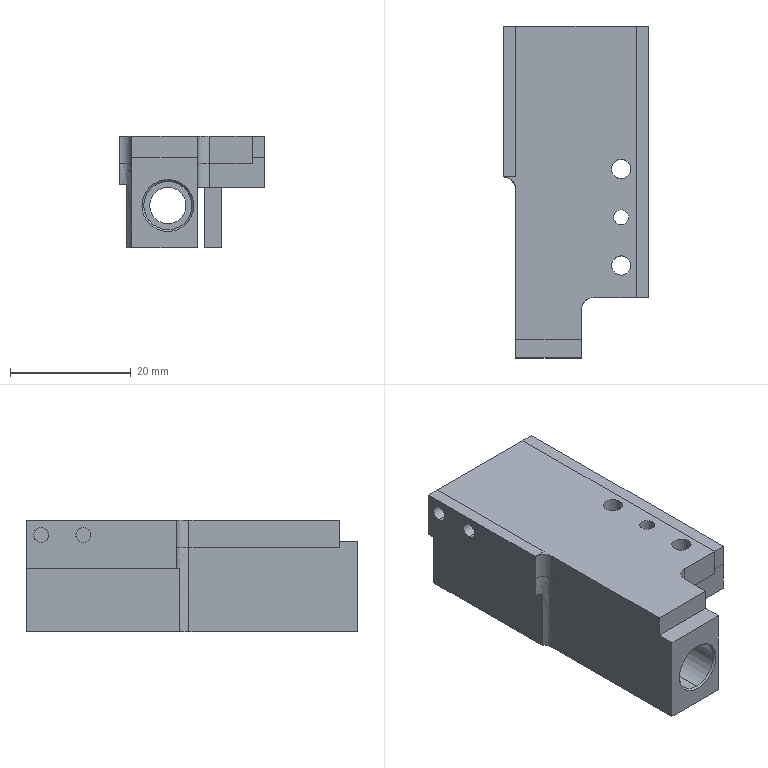NC program | NX | posted with a generic post | part box 24.15 x 55 x 18.5 mm
Whole program:
N10 G17 G21 G94 G90
(FLOOR_WALL_1_COPY_1_COPY , TOOL : D10)
N12 T10 M6
N14 G54
N16 G17 G0 G90 X18.075 Y6.103 B0. C0. S9500 M3
N18 G43 Z30. H10
N20 Z-0.85
N22 G94 G1 X17.575 Y5.815 F1000.
N24 G3 X17.075 Y4.949 R1.
N26 G1 Y-22.603 F3000.
N28 X6.003
N30 Y-32.5
N32 X-15.103
N34 Y-2.6
N36 X-4.9
N38 Y32.5
N40 X17.075
N42 Y4.949
N44 X12.075
N46 Y-17.603
N48 X6.003
N50 G3 X1.003 Y-22.603 R5.
N52 G1 Y-27.5
N54 X-10.103
N56 Y-7.6
N58 X-4.9
N60 G3 X0.1 Y-2.6 R5.
N62 G1 Y27.5
N64 X12.075
N66 Y4.949
N68 X7.075
N70 Y-12.603
N72 X6.003
N74 G3 X-3.996 Y-22.5 R10.
N76 G1 X-5.103
N78 Y-12.6
N80 G3 X5.1 Y-2.6 R10.
N82 G1 Y22.5
N84 X7.075
N86 Y4.949
N88 G3 X7.575 Y4.082 R1.
N90 G0 Z30.
N92 X18.075 Y6.103
N94 Z-1.7
N96 G1 X17.575 Y5.815 F1000.
N98 G3 X17.075 Y4.949 R1.
N100 G1 Y-22.603 F3000.
N102 X6.003
N104 Y-32.5
N106 X-15.103
N108 Y-2.6
N110 X-4.9
N112 Y32.5
N114 X17.075
N116 Y4.949
N118 X12.075
N120 Y-17.603
N122 X6.003
N124 G3 X1.003 Y-22.603 R5.
N126 G1 Y-27.5
N128 X-10.103
N130 Y-7.6
N132 X-4.9
N134 G3 X0.1 Y-2.6 R5.
N136 G1 Y27.5
N138 X12.075
N140 Y4.949
N142 X7.075
N144 Y-12.603
N146 X6.003
N148 G3 X-3.996 Y-22.5 R10.
N150 G1 X-5.103
N152 Y-12.6
N154 G3 X5.1 Y-2.6 R10.
N156 G1 Y22.5
N158 X7.075
N160 Y4.949
N162 G3 X7.575 Y4.082 R1.
N164 G0 Z30.
N166 X18.075 Y6.103
N168 Z-2.55
N170 G1 X17.575 Y5.815 F1000.
N172 G3 X17.075 Y4.949 R1.
N174 G1 Y-22.603 F3000.
N176 X6.003
N178 Y-32.5
N180 X-15.103
N182 Y-2.6
N184 X-4.9
N186 Y32.5
N188 X17.075
N190 Y4.949
N192 X12.075
N194 Y-17.603
N196 X6.003
N198 G3 X1.003 Y-22.603 R5.
N200 G1 Y-27.5
N202 X-10.103
N204 Y-7.6
N206 X-4.9
N208 G3 X0.1 Y-2.6 R5.
N210 G1 Y27.5
N212 X12.075
N214 Y4.949
N216 X7.075
N218 Y-12.603
N220 X6.003
N222 G3 X-3.996 Y-22.5 R10.
N224 G1 X-5.103
N226 Y-12.6
N228 G3 X5.1 Y-2.6 R10.
N230 G1 Y22.5
N232 X7.075
N234 Y4.949
N236 G3 X7.575 Y4.082 R1.
N238 G0 Z30.
N240 X18.075 Y6.103
N242 Z-3.4
N244 G1 X17.575 Y5.815 F1000.
N246 G3 X17.075 Y4.949 R1.
N248 G1 Y-22.603 F3000.
N250 X6.003
N252 Y-32.5
N254 X-15.103
N256 Y-2.6
N258 X-4.9
N260 Y32.5
N262 X17.075
N264 Y4.949
N266 X12.075
N268 Y-17.603
N270 X6.003
N272 G3 X1.003 Y-22.603 R5.
N274 G1 Y-27.5
N276 X-10.103
N278 Y-7.6
N280 X-4.9
N282 G3 X0.1 Y-2.6 R5.
N284 G1 Y27.5
N286 X12.075
N288 Y4.949
N290 X7.075
N292 Y-12.603
N294 X6.003
N296 G3 X-3.996 Y-22.5 R10.
N298 G1 X-5.103
N300 Y-12.6
N302 G3 X5.1 Y-2.6 R10.
N304 G1 Y22.5
N306 X7.075
N308 Y4.949
N310 G3 X7.575 Y4.082 R1.
N312 G0 Z30.
N314 X-18.075 Y-11.866
N316 Z-4.4
N318 G1 X-15.603 F1000.
N320 G3 X-15.103 Y-11. R1.
N322 G1 Y-2.6 F3000.
N324 X-10.103
N326 X-4.9
N328 Y32.5
N330 X4.9
N332 Y-19.4
N334 X-15.103
N336 Y-11.
N338 X-10.103
N340 Y-7.6
N342 X-4.9
N344 G3 X-0.1 Y-4.001 R5.
N346 G1 Y-14.4
N348 X-10.103
N350 Y-11.
N352 G3 X-10.603 Y-10.134 R1.
N354 G0 Z30.
N356 M5
(FLOOR_WALL_1_COPY_COPY_1 , TOOL : D6)
N358 T06 M6
N360 G54
N362 G17 G0 G90 X6.324 Y-21.237 B0. C0. S9500 M3
N364 G43 Z30. H6
N366 Z-3.5
N368 G94 G1 X6.7 Y-21.02 F1000.
N370 G3 X7. Y-20.5 R0.6
N372 G1 Y30.5 F1500.
N374 X9.675
N376 Y-20.5
N378 G2 X9.375 Y-21.02 R0.6
N380 G1 X8.543 Y-21.5
N382 G0 Z30.
N384 X6.397 Y31.5
N386 Z-4.5
N388 G1 Y29.98 F1000.
N390 G3 X6.697 Y30.5 R0.6
N392 G1 Y-20.5 F1500.
N394 X3.9
N396 Y-21.202
N398 X3.87 Y-21.2
N400 X3.838
N402 Y30.5
N404 X0.978
N406 Y-21.2
N408 X-1.881
N410 Y30.5
N412 X-4.741
N414 Y-21.2
N416 X-7.6
N418 Y-0.8
N420 X-10.459
N422 Y-21.2
N424 G3 X-9.94 Y-20.9 R0.6
N426 G1 X-14. Y-20.368
N428 X-13.52 Y-21.2 F1000.
N430 G3 X-13. Y-21.5 R0.6
N432 G1 X3.87 F1500.
N434 G3 X4.39 Y-21.2 R0.6
N436 G1 X6.7 Y-21.02
N438 G3 X7. Y-20.5 R0.6 F1000.
N440 G1 Y30.5 F1500.
N442 G3 X6.7 Y31.02 R0.6
N444 G1 X5.868 Y31.5
N446 X-5.868
N448 X-6.7 Y31.02 F1000.
N450 G3 X-7. Y30.5 R0.6
N452 G1 Y-0.5 F1500.
N454 X-13.
N456 G3 X-13.52 Y-0.8 R0.6
N458 G1 X-14. Y-1.632
N460 G0 Z30.
N462 M5
(PLANAR_MILL_COPY_1 , TOOL : D6A45)
N464 T07 M6
N466 G54
N468 G17 G0 G90 X-13.382 Y14.234 B0. C0. S9500 M3
N470 G43 Z30. H7
N472 Z2.
N474 G94 G1 Z-1. F1250.
N476 G3 X-13.025 Y15. R1.
N478 G1 Y27.5
N480 G2 X-12.075 Y28.45 R0.95
N482 G1 X-10.
N484 G2 X-9.05 Y27.5 R0.95
N486 G1 Y2.5
N488 G2 X-10. Y1.55 R0.95
N490 G1 X-12.075
N492 G2 X-13.025 Y2.5 R0.95
N494 G1 Y15.
N496 G3 X-13.382 Y15.766 R1.
N498 G1 Z2.
N500 G0 Z30.
(PLANAR_MILL_COPY_1_COPY , TOOL : D6A45)
N502 X12.982 Y5.766
N504 Z-1.1
N506 G1 Z-4.1
N508 G3 X12.625 Y5. R1.
N510 G1 Y-17.5
N512 G2 X12.075 Y-18.05 R0.55
N514 G1 X10.
N516 G2 X9.45 Y-17.5 R0.55
N518 G1 Y27.5
N520 G2 X10. Y28.05 R0.55
N522 G1 X12.075
N524 G2 X12.625 Y27.5 R0.55
N526 G1 Y5.
N528 G3 X12.982 Y4.234 R1.
N530 G1 Z-1.1
N532 G0 Z30.
N534 X-3.784 Y-28.407
N536 Z-1.1
N538 G1 Z-4.1
N540 G3 X-4.55 Y-28.05 R1.
N542 G1 X-10.
N544 G2 X-10.55 Y-27.5 R0.55
N546 G1 Y-24.5
N548 G2 X-10. Y-23.95 R0.55
N550 G1 X0.9
N552 G2 X1.45 Y-24.5 R0.55
N554 G1 Y-27.5
N556 G2 X0.9 Y-28.05 R0.55
N558 G1 X-4.55
N560 G3 X-5.316 Y-28.407 R1.
N562 G1 Z-1.1
N564 G0 Z30.
(PLANAR_MILL_COPY_1_COPY_1 , TOOL : D6A45)
N566 X7.223 Y-19.945
N568 Z-2.5
N570 G1 Z-5.5
N572 X7.61 Y-19.243
N574 G3 X7.668 Y-18.4 R1.
N576 G1 X2.9
N578 G3 X1.8 Y-19.5 R1.1
N580 G1 Y-22.168
N582 G3 X2.643 Y-22.11 R1.
N584 G1 X3.345 Y-21.723
N586 Z-2.5
N588 G0 Z30.
N590 X-12.445
N592 Z-2.5
N594 G1 Z-5.5
N596 X-11.743 Y-22.11
N598 G3 X-10.9 Y-22.168 R1.
N600 G1 Y-1.
N602 G3 X-11.666 Y-1.357 R1.
N604 G1 X-12.366 Y-2.191
N606 Z-2.5
N608 G0 Z30.
N610 X-5.978 Y29.932
N612 Z-2.5
N614 G1 Z-5.5
N616 X-6.469 Y29.232
N618 G3 X-6.618 Y28.4 R1.
N620 G1 X7.668
N622 G3 X7.61 Y29.243 R1.
N624 G1 X7.223 Y29.945
N626 Z-2.5
N628 G0 Z30.
N630 M5
N632 M2